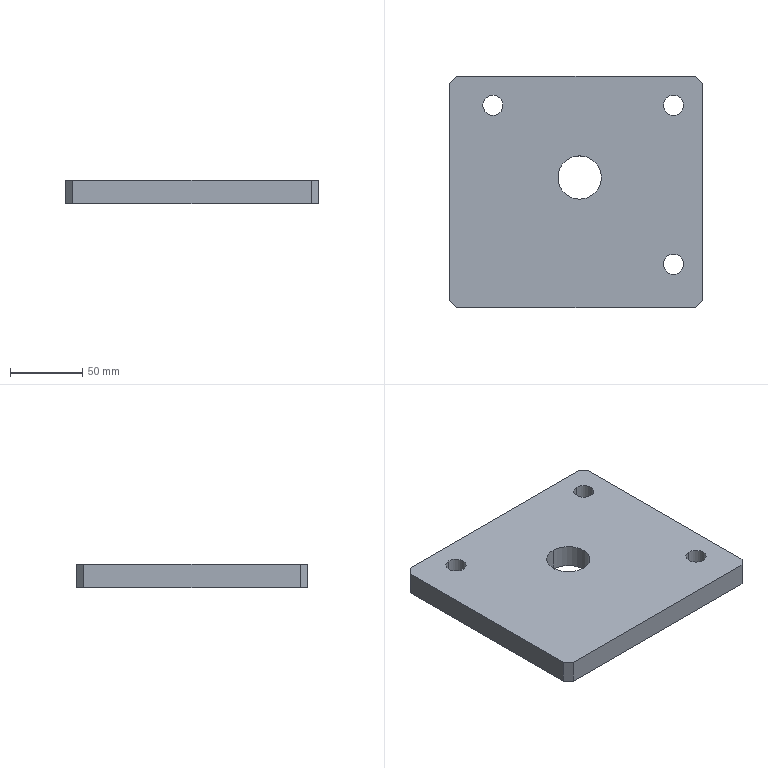Part | STEP file | [03]-1 | 1 solid | 18 faces | box 175 x 160 x 16 mm | volume 428501 mm3 | plane 10 | cylinder 8 | commonest cylinder face diameters 14 x6 30 x2